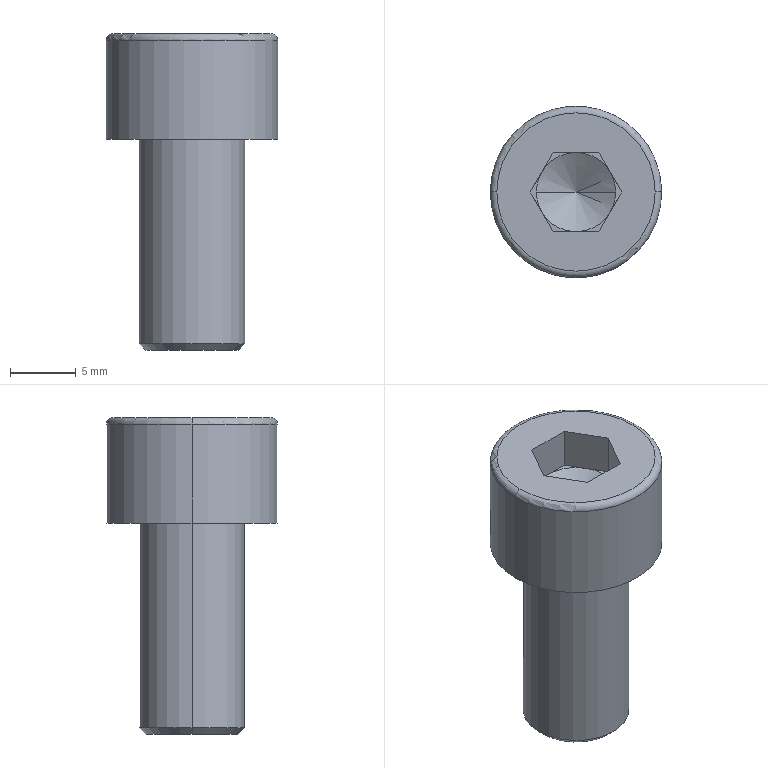Part | NX | features BREP 1 | 1 solid | 25 faces | box 13 x 13 x 24 mm | volume 1747 mm3 | plane 15 | cone 4 | cylinder 4 | torus 2 | commonest cylinder face diameters 8 x2 13 x2
STEP:
#1=CARTESIAN_POINT('',(0.,0.,3.148));
#2=VERTEX_POINT('',#1);
#3=CARTESIAN_POINT('',(-3.,0.,4.88));
#4=VERTEX_POINT('',#3);
#5=CARTESIAN_POINT('',(-3.,0.,4.88));
#6=DIRECTION('',(-0.866,0.,0.5));
#7=VECTOR('',#6,1000.);
#8=LINE('',#5,#7);
#9=EDGE_CURVE('',#2,#4,#8,.T.);
#10=ORIENTED_EDGE('',*,*,#9,.F.);
#11=CARTESIAN_POINT('',(3.,0.,4.88));
#12=VERTEX_POINT('',#11);
#13=CARTESIAN_POINT('',(3.,0.,4.88));
#14=DIRECTION('',(0.866,0.,0.5));
#15=VECTOR('',#14,1000.);
#16=LINE('',#13,#15);
#17=EDGE_CURVE('',#2,#12,#16,.T.);
#18=ORIENTED_EDGE('',*,*,#17,.T.);
#19=CARTESIAN_POINT('',(2.598,1.5,4.88));
#20=VERTEX_POINT('',#19);
#21=CARTESIAN_POINT('',(0.,0.,4.88));
#22=DIRECTION('',(0.,0.,1.));
#23=DIRECTION('',(1.,0.,0.));
#24=AXIS2_PLACEMENT_3D('',#21,#22,#23);
#25=CIRCLE('',#24,3.);
#26=EDGE_CURVE('',#12,#20,#25,.T.);
#27=ORIENTED_EDGE('',*,*,#26,.T.);
#28=CARTESIAN_POINT('',(0.,3.,4.88));
#29=VERTEX_POINT('',#28);
#30=CARTESIAN_POINT('',(0.,0.,4.88));
#31=DIRECTION('',(0.,0.,1.));
#32=DIRECTION('',(1.,0.,0.));
#33=AXIS2_PLACEMENT_3D('',#30,#31,#32);
#34=CIRCLE('',#33,3.);
#35=EDGE_CURVE('',#20,#29,#34,.T.);
#36=ORIENTED_EDGE('',*,*,#35,.T.);
#37=CARTESIAN_POINT('',(-2.598,1.5,4.88));
#38=VERTEX_POINT('',#37);
#39=CARTESIAN_POINT('',(0.,0.,4.88));
#40=DIRECTION('',(0.,0.,-1.));
#41=DIRECTION('',(-1.,0.,0.));
#42=AXIS2_PLACEMENT_3D('',#39,#40,#41);
#43=CIRCLE('',#42,3.);
#44=EDGE_CURVE('',#38,#29,#43,.T.);
#45=ORIENTED_EDGE('',*,*,#44,.F.);
#46=CARTESIAN_POINT('',(0.,0.,4.88));
#47=DIRECTION('',(0.,0.,1.));
#48=DIRECTION('',(1.,0.,0.));
#49=AXIS2_PLACEMENT_3D('',#46,#47,#48);
#50=CIRCLE('',#49,3.);
#51=EDGE_CURVE('',#38,#4,#50,.T.);
#52=ORIENTED_EDGE('',*,*,#51,.T.);
#53=EDGE_LOOP('',(#10,#18,#27,#36,#45,#52));
#54=FACE_BOUND('',#53,.T.);
#55=CARTESIAN_POINT('',(0.,0.,4.88));
#56=DIRECTION('',(0.,0.,1.));
#57=DIRECTION('',(-1.,0.,0.));
#58=AXIS2_PLACEMENT_3D('',#55,#56,#57);
#59=CONICAL_SURFACE('',#58,3.,1.047);
#60=ADVANCED_FACE('',(#54),#59,.F.);
#61=CARTESIAN_POINT('',(-3.5,0.,-16.));
#62=VERTEX_POINT('',#61);
#63=CARTESIAN_POINT('',(3.5,0.,-16.));
#64=VERTEX_POINT('',#63);
#65=CARTESIAN_POINT('',(0.,0.,-16.));
#66=DIRECTION('',(0.,0.,1.));
#67=DIRECTION('',(-1.,0.,0.));
#68=AXIS2_PLACEMENT_3D('',#65,#66,#67);
#69=CIRCLE('',#68,3.5);
#70=EDGE_CURVE('',#62,#64,#69,.T.);
#71=ORIENTED_EDGE('',*,*,#70,.T.);
#72=CARTESIAN_POINT('',(4.,0.,-15.5));
#73=VERTEX_POINT('',#72);
#74=CARTESIAN_POINT('',(4.,0.,-15.5));
#75=DIRECTION('',(0.7071,0.,0.7071));
#76=VECTOR('',#75,1000.);
#77=LINE('',#74,#76);
#78=EDGE_CURVE('',#64,#73,#77,.T.);
#79=ORIENTED_EDGE('',*,*,#78,.T.);
#80=CARTESIAN_POINT('',(-4.,0.,-15.5));
#81=VERTEX_POINT('',#80);
#82=CARTESIAN_POINT('',(0.,0.,-15.5));
#83=DIRECTION('',(0.,0.,-1.));
#84=DIRECTION('',(-1.,0.,0.));
#85=AXIS2_PLACEMENT_3D('',#82,#83,#84);
#86=CIRCLE('',#85,4.);
#87=EDGE_CURVE('',#73,#81,#86,.T.);
#88=ORIENTED_EDGE('',*,*,#87,.T.);
#89=CARTESIAN_POINT('',(-4.,0.,-15.5));
#90=DIRECTION('',(-0.7071,0.,0.7071));
#91=VECTOR('',#90,1000.);
#92=LINE('',#89,#91);
#93=EDGE_CURVE('',#62,#81,#92,.T.);
#94=ORIENTED_EDGE('',*,*,#93,.F.);
#95=EDGE_LOOP('',(#71,#79,#88,#94));
#96=FACE_BOUND('',#95,.T.);
#97=CARTESIAN_POINT('',(0.,0.,-15.5));
#98=DIRECTION('',(0.,0.,1.));
#99=DIRECTION('',(-1.,0.,0.));
#100=AXIS2_PLACEMENT_3D('',#97,#98,#99);
#101=CONICAL_SURFACE('',#100,4.,0.7854);
#102=ADVANCED_FACE('',(#96),#101,.T.);
#103=CARTESIAN_POINT('',(6.,0.,8.));
#104=VERTEX_POINT('',#103);
#105=CARTESIAN_POINT('',(-6.,0.,8.));
#106=VERTEX_POINT('',#105);
#107=CARTESIAN_POINT('',(0.,0.,8.));
#108=DIRECTION('',(0.,0.,-1.));
#109=DIRECTION('',(1.,0.,0.));
#110=AXIS2_PLACEMENT_3D('',#107,#108,#109);
#111=CIRCLE('',#110,6.);
#112=EDGE_CURVE('',#104,#106,#111,.T.);
#113=ORIENTED_EDGE('',*,*,#112,.T.);
#114=CARTESIAN_POINT('',(-6.5,0.,7.5));
#115=VERTEX_POINT('',#114);
#116=CARTESIAN_POINT('',(-6.,0.,7.5));
#117=DIRECTION('',(0.,-1.,0.));
#118=DIRECTION('',(1.,0.,0.));
#119=AXIS2_PLACEMENT_3D('',#116,#117,#118);
#120=CIRCLE('',#119,0.5);
#121=EDGE_CURVE('',#115,#106,#120,.F.);
#122=ORIENTED_EDGE('',*,*,#121,.F.);
#123=CARTESIAN_POINT('',(6.5,0.,7.5));
#124=VERTEX_POINT('',#123);
#125=CARTESIAN_POINT('',(0.,0.,7.5));
#126=DIRECTION('',(0.,0.,1.));
#127=DIRECTION('',(1.,0.,0.));
#128=AXIS2_PLACEMENT_3D('',#125,#126,#127);
#129=CIRCLE('',#128,6.5);
#130=EDGE_CURVE('',#115,#124,#129,.T.);
#131=ORIENTED_EDGE('',*,*,#130,.T.);
#132=CARTESIAN_POINT('',(6.,0.,7.5));
#133=DIRECTION('',(0.,1.,0.));
#134=DIRECTION('',(0.,0.,1.));
#135=AXIS2_PLACEMENT_3D('',#132,#133,#134);
#136=CIRCLE('',#135,0.5);
#137=EDGE_CURVE('',#124,#104,#136,.F.);
#138=ORIENTED_EDGE('',*,*,#137,.T.);
#139=EDGE_LOOP('',(#113,#122,#131,#138));
#140=FACE_BOUND('',#139,.T.);
#141=CARTESIAN_POINT('',(0.,0.,7.5));
#142=DIRECTION('',(0.,0.,-1.));
#143=DIRECTION('',(1.,0.,0.));
#144=AXIS2_PLACEMENT_3D('',#141,#142,#143);
#145=TOROIDAL_SURFACE('',#144,6.,0.5);
#146=ADVANCED_FACE('',(#140),#145,.T.);
#147=ORIENTED_EDGE('',*,*,#87,.F.);
#148=CARTESIAN_POINT('',(4.,0.,0.));
#149=VERTEX_POINT('',#148);
#150=CARTESIAN_POINT('',(4.,0.,-16.));
#151=DIRECTION('',(0.,0.,1.));
#152=VECTOR('',#151,1000.);
#153=LINE('',#150,#152);
#154=EDGE_CURVE('',#73,#149,#153,.T.);
#155=ORIENTED_EDGE('',*,*,#154,.T.);
#156=CARTESIAN_POINT('',(-4.,0.,0.));
#157=VERTEX_POINT('',#156);
#158=CARTESIAN_POINT('',(0.,0.,0.));
#159=DIRECTION('',(0.,0.,1.));
#160=DIRECTION('',(1.,0.,0.));
#161=AXIS2_PLACEMENT_3D('',#158,#159,#160);
#162=CIRCLE('',#161,4.);
#163=EDGE_CURVE('',#157,#149,#162,.T.);
#164=ORIENTED_EDGE('',*,*,#163,.F.);
#165=CARTESIAN_POINT('',(-4.,0.,-16.));
#166=DIRECTION('',(0.,0.,1.));
#167=VECTOR('',#166,1000.);
#168=LINE('',#165,#167);
#169=EDGE_CURVE('',#81,#157,#168,.T.);
#170=ORIENTED_EDGE('',*,*,#169,.F.);
#171=EDGE_LOOP('',(#147,#155,#164,#170));
#172=FACE_BOUND('',#171,.T.);
#173=CARTESIAN_POINT('',(0.,0.,-16.));
#174=DIRECTION('',(0.,0.,1.));
#175=DIRECTION('',(-1.,0.,0.));
#176=AXIS2_PLACEMENT_3D('',#173,#174,#175);
#177=CYLINDRICAL_SURFACE('',#176,4.);
#178=ADVANCED_FACE('',(#172),#177,.T.);
#179=ORIENTED_EDGE('',*,*,#130,.F.);
#180=CARTESIAN_POINT('',(-6.5,0.,0.));
#181=VERTEX_POINT('',#180);
#182=CARTESIAN_POINT('',(-6.5,0.,8.));
#183=DIRECTION('',(0.,0.,-1.));
#184=VECTOR('',#183,1000.);
#185=LINE('',#182,#184);
#186=EDGE_CURVE('',#181,#115,#185,.F.);
#187=ORIENTED_EDGE('',*,*,#186,.F.);
#188=CARTESIAN_POINT('',(6.5,0.,0.));
#189=VERTEX_POINT('',#188);
#190=CARTESIAN_POINT('',(0.,0.,0.));
#191=DIRECTION('',(0.,0.,1.));
#192=DIRECTION('',(1.,0.,0.));
#193=AXIS2_PLACEMENT_3D('',#190,#191,#192);
#194=CIRCLE('',#193,6.5);
#195=EDGE_CURVE('',#181,#189,#194,.T.);
#196=ORIENTED_EDGE('',*,*,#195,.T.);
#197=CARTESIAN_POINT('',(6.5,0.,8.));
#198=DIRECTION('',(0.,0.,-1.));
#199=VECTOR('',#198,1000.);
#200=LINE('',#197,#199);
#201=EDGE_CURVE('',#189,#124,#200,.F.);
#202=ORIENTED_EDGE('',*,*,#201,.T.);
#203=EDGE_LOOP('',(#179,#187,#196,#202));
#204=FACE_BOUND('',#203,.T.);
#205=CARTESIAN_POINT('',(0.,0.,8.));
#206=DIRECTION('',(0.,0.,-1.));
#207=DIRECTION('',(1.,0.,0.));
#208=AXIS2_PLACEMENT_3D('',#205,#206,#207);
#209=CYLINDRICAL_SURFACE('',#208,6.5);
#210=ADVANCED_FACE('',(#204),#209,.T.);
#211=CARTESIAN_POINT('',(1.732,3.,4.88));
#212=VERTEX_POINT('',#211);
#213=CARTESIAN_POINT('',(3.464,0.,4.88));
#214=DIRECTION('',(-0.5,0.866,0.));
#215=VECTOR('',#214,1000.);
#216=LINE('',#213,#215);
#217=EDGE_CURVE('',#20,#212,#216,.T.);
#218=ORIENTED_EDGE('',*,*,#217,.T.);
#219=CARTESIAN_POINT('',(1.732,3.,4.88));
#220=DIRECTION('',(-1.,0.,0.));
#221=VECTOR('',#220,1000.);
#222=LINE('',#219,#221);
#223=EDGE_CURVE('',#212,#29,#222,.T.);
#224=ORIENTED_EDGE('',*,*,#223,.T.);
#225=ORIENTED_EDGE('',*,*,#35,.F.);
#226=EDGE_LOOP('',(#218,#224,#225));
#227=FACE_BOUND('',#226,.T.);
#228=CARTESIAN_POINT('',(0.,0.,4.88));
#229=DIRECTION('',(0.,0.,-1.));
#230=DIRECTION('',(0.,-1.,0.));
#231=AXIS2_PLACEMENT_3D('',#228,#229,#230);
#232=PLANE('',#231);
#233=ADVANCED_FACE('',(#227),#232,.F.);
#234=CARTESIAN_POINT('',(-1.732,3.,4.88));
#235=VERTEX_POINT('',#234);
#236=CARTESIAN_POINT('',(1.732,3.,4.88));
#237=DIRECTION('',(-1.,0.,0.));
#238=VECTOR('',#237,1000.);
#239=LINE('',#236,#238);
#240=EDGE_CURVE('',#29,#235,#239,.T.);
#241=ORIENTED_EDGE('',*,*,#240,.T.);
#242=CARTESIAN_POINT('',(-1.732,3.,4.88));
#243=DIRECTION('',(-0.5,-0.866,0.));
#244=VECTOR('',#243,1000.);
#245=LINE('',#242,#244);
#246=EDGE_CURVE('',#235,#38,#245,.T.);
#247=ORIENTED_EDGE('',*,*,#246,.T.);
#248=ORIENTED_EDGE('',*,*,#44,.T.);
#249=EDGE_LOOP('',(#241,#247,#248));
#250=FACE_BOUND('',#249,.T.);
#251=CARTESIAN_POINT('',(0.,0.,4.88));
#252=DIRECTION('',(0.,0.,-1.));
#253=DIRECTION('',(0.,-1.,0.));
#254=AXIS2_PLACEMENT_3D('',#251,#252,#253);
#255=PLANE('',#254);
#256=ADVANCED_FACE('',(#250),#255,.F.);
#257=CARTESIAN_POINT('',(-3.464,0.,4.88));
#258=VERTEX_POINT('',#257);
#259=CARTESIAN_POINT('',(-1.732,3.,4.88));
#260=DIRECTION('',(-0.5,-0.866,0.));
#261=VECTOR('',#260,1000.);
#262=LINE('',#259,#261);
#263=EDGE_CURVE('',#38,#258,#262,.T.);
#264=ORIENTED_EDGE('',*,*,#263,.T.);
#265=CARTESIAN_POINT('',(-2.598,-1.5,4.88));
#266=VERTEX_POINT('',#265);
#267=CARTESIAN_POINT('',(-3.464,0.,4.88));
#268=DIRECTION('',(0.5,-0.866,0.));
#269=VECTOR('',#268,1000.);
#270=LINE('',#267,#269);
#271=EDGE_CURVE('',#258,#266,#270,.T.);
#272=ORIENTED_EDGE('',*,*,#271,.T.);
#273=CARTESIAN_POINT('',(0.,0.,4.88));
#274=DIRECTION('',(0.,0.,1.));
#275=DIRECTION('',(1.,0.,0.));
#276=AXIS2_PLACEMENT_3D('',#273,#274,#275);
#277=CIRCLE('',#276,3.);
#278=EDGE_CURVE('',#4,#266,#277,.T.);
#279=ORIENTED_EDGE('',*,*,#278,.F.);
#280=ORIENTED_EDGE('',*,*,#51,.F.);
#281=EDGE_LOOP('',(#264,#272,#279,#280));
#282=FACE_BOUND('',#281,.T.);
#283=CARTESIAN_POINT('',(0.,0.,4.88));
#284=DIRECTION('',(0.,0.,-1.));
#285=DIRECTION('',(0.,-1.,0.));
#286=AXIS2_PLACEMENT_3D('',#283,#284,#285);
#287=PLANE('',#286);
#288=ADVANCED_FACE('',(#282),#287,.F.);
#289=CARTESIAN_POINT('',(-1.732,-3.,4.88));
#290=VERTEX_POINT('',#289);
#291=CARTESIAN_POINT('',(-3.464,0.,4.88));
#292=DIRECTION('',(0.5,-0.866,0.));
#293=VECTOR('',#292,1000.);
#294=LINE('',#291,#293);
#295=EDGE_CURVE('',#266,#290,#294,.T.);
#296=ORIENTED_EDGE('',*,*,#295,.T.);
#297=CARTESIAN_POINT('',(0.,-3.,4.88));
#298=VERTEX_POINT('',#297);
#299=CARTESIAN_POINT('',(-1.732,-3.,4.88));
#300=DIRECTION('',(1.,0.,0.));
#301=VECTOR('',#300,1000.);
#302=LINE('',#299,#301);
#303=EDGE_CURVE('',#290,#298,#302,.T.);
#304=ORIENTED_EDGE('',*,*,#303,.T.);
#305=CARTESIAN_POINT('',(0.,0.,4.88));
#306=DIRECTION('',(0.,0.,1.));
#307=DIRECTION('',(1.,0.,0.));
#308=AXIS2_PLACEMENT_3D('',#305,#306,#307);
#309=CIRCLE('',#308,3.);
#310=EDGE_CURVE('',#266,#298,#309,.T.);
#311=ORIENTED_EDGE('',*,*,#310,.F.);
#312=EDGE_LOOP('',(#296,#304,#311));
#313=FACE_BOUND('',#312,.T.);
#314=CARTESIAN_POINT('',(0.,0.,4.88));
#315=DIRECTION('',(0.,0.,-1.));
#316=DIRECTION('',(0.,-1.,0.));
#317=AXIS2_PLACEMENT_3D('',#314,#315,#316);
#318=PLANE('',#317);
#319=ADVANCED_FACE('',(#313),#318,.F.);
#320=CARTESIAN_POINT('',(1.732,-3.,4.88));
#321=VERTEX_POINT('',#320);
#322=CARTESIAN_POINT('',(-1.732,-3.,4.88));
#323=DIRECTION('',(1.,0.,0.));
#324=VECTOR('',#323,1000.);
#325=LINE('',#322,#324);
#326=EDGE_CURVE('',#298,#321,#325,.T.);
#327=ORIENTED_EDGE('',*,*,#326,.T.);
#328=CARTESIAN_POINT('',(2.598,-1.5,4.88));
#329=VERTEX_POINT('',#328);
#330=CARTESIAN_POINT('',(1.732,-3.,4.88));
#331=DIRECTION('',(0.5,0.866,0.));
#332=VECTOR('',#331,1000.);
#333=LINE('',#330,#332);
#334=EDGE_CURVE('',#321,#329,#333,.T.);
#335=ORIENTED_EDGE('',*,*,#334,.T.);
#336=CARTESIAN_POINT('',(0.,0.,4.88));
#337=DIRECTION('',(0.,0.,1.));
#338=DIRECTION('',(1.,0.,0.));
#339=AXIS2_PLACEMENT_3D('',#336,#337,#338);
#340=CIRCLE('',#339,3.);
#341=EDGE_CURVE('',#298,#329,#340,.T.);
#342=ORIENTED_EDGE('',*,*,#341,.F.);
#343=EDGE_LOOP('',(#327,#335,#342));
#344=FACE_BOUND('',#343,.T.);
#345=CARTESIAN_POINT('',(0.,0.,4.88));
#346=DIRECTION('',(0.,0.,-1.));
#347=DIRECTION('',(0.,-1.,0.));
#348=AXIS2_PLACEMENT_3D('',#345,#346,#347);
#349=PLANE('',#348);
#350=ADVANCED_FACE('',(#344),#349,.F.);
#351=ORIENTED_EDGE('',*,*,#112,.F.);
#352=CARTESIAN_POINT('',(0.,0.,8.));
#353=DIRECTION('',(0.,0.,-1.));
#354=DIRECTION('',(1.,0.,0.));
#355=AXIS2_PLACEMENT_3D('',#352,#353,#354);
#356=CIRCLE('',#355,6.);
#357=EDGE_CURVE('',#106,#104,#356,.T.);
#358=ORIENTED_EDGE('',*,*,#357,.F.);
#359=EDGE_LOOP('',(#351,#358));
#360=FACE_BOUND('',#359,.T.);
#361=CARTESIAN_POINT('',(3.464,0.,8.));
#362=VERTEX_POINT('',#361);
#363=CARTESIAN_POINT('',(1.732,3.,8.));
#364=VERTEX_POINT('',#363);
#365=CARTESIAN_POINT('',(3.464,0.,8.));
#366=DIRECTION('',(-0.5,0.866,0.));
#367=VECTOR('',#366,1000.);
#368=LINE('',#365,#367);
#369=EDGE_CURVE('',#362,#364,#368,.T.);
#370=ORIENTED_EDGE('',*,*,#369,.F.);
#371=CARTESIAN_POINT('',(1.732,-3.,8.));
#372=VERTEX_POINT('',#371);
#373=CARTESIAN_POINT('',(1.732,-3.,8.));
#374=DIRECTION('',(0.5,0.866,0.));
#375=VECTOR('',#374,1000.);
#376=LINE('',#373,#375);
#377=EDGE_CURVE('',#372,#362,#376,.T.);
#378=ORIENTED_EDGE('',*,*,#377,.F.);
#379=CARTESIAN_POINT('',(-1.732,-3.,8.));
#380=VERTEX_POINT('',#379);
#381=CARTESIAN_POINT('',(-1.732,-3.,8.));
#382=DIRECTION('',(1.,0.,0.));
#383=VECTOR('',#382,1000.);
#384=LINE('',#381,#383);
#385=EDGE_CURVE('',#380,#372,#384,.T.);
#386=ORIENTED_EDGE('',*,*,#385,.F.);
#387=CARTESIAN_POINT('',(-3.464,0.,8.));
#388=VERTEX_POINT('',#387);
#389=CARTESIAN_POINT('',(-3.464,0.,8.));
#390=DIRECTION('',(0.5,-0.866,0.));
#391=VECTOR('',#390,1000.);
#392=LINE('',#389,#391);
#393=EDGE_CURVE('',#388,#380,#392,.T.);
#394=ORIENTED_EDGE('',*,*,#393,.F.);
#395=CARTESIAN_POINT('',(-1.732,3.,8.));
#396=VERTEX_POINT('',#395);
#397=CARTESIAN_POINT('',(-1.732,3.,8.));
#398=DIRECTION('',(-0.5,-0.866,0.));
#399=VECTOR('',#398,1000.);
#400=LINE('',#397,#399);
#401=EDGE_CURVE('',#396,#388,#400,.T.);
#402=ORIENTED_EDGE('',*,*,#401,.F.);
#403=CARTESIAN_POINT('',(1.732,3.,8.));
#404=DIRECTION('',(-1.,0.,0.));
#405=VECTOR('',#404,1000.);
#406=LINE('',#403,#405);
#407=EDGE_CURVE('',#364,#396,#406,.T.);
#408=ORIENTED_EDGE('',*,*,#407,.F.);
#409=EDGE_LOOP('',(#370,#378,#386,#394,#402,#408));
#410=FACE_BOUND('',#409,.T.);
#411=CARTESIAN_POINT('',(0.,0.,8.));
#412=DIRECTION('',(0.,0.,-1.));
#413=DIRECTION('',(0.,-1.,0.));
#414=AXIS2_PLACEMENT_3D('',#411,#412,#413);
#415=PLANE('',#414);
#416=ADVANCED_FACE('',(#360,#410),#415,.F.);
#417=ORIENTED_EDGE('',*,*,#186,.T.);
#418=CARTESIAN_POINT('',(0.,0.,7.5));
#419=DIRECTION('',(0.,0.,1.));
#420=DIRECTION('',(1.,0.,0.));
#421=AXIS2_PLACEMENT_3D('',#418,#419,#420);
#422=CIRCLE('',#421,6.5);
#423=EDGE_CURVE('',#124,#115,#422,.T.);
#424=ORIENTED_EDGE('',*,*,#423,.F.);
#425=ORIENTED_EDGE('',*,*,#201,.F.);
#426=CARTESIAN_POINT('',(0.,0.,0.));
#427=DIRECTION('',(0.,0.,1.));
#428=DIRECTION('',(1.,0.,0.));
#429=AXIS2_PLACEMENT_3D('',#426,#427,#428);
#430=CIRCLE('',#429,6.5);
#431=EDGE_CURVE('',#189,#181,#430,.T.);
#432=ORIENTED_EDGE('',*,*,#431,.T.);
#433=EDGE_LOOP('',(#417,#424,#425,#432));
#434=FACE_BOUND('',#433,.T.);
#435=CARTESIAN_POINT('',(0.,0.,8.));
#436=DIRECTION('',(0.,0.,-1.));
#437=DIRECTION('',(1.,0.,0.));
#438=AXIS2_PLACEMENT_3D('',#435,#436,#437);
#439=CYLINDRICAL_SURFACE('',#438,6.5);
#440=ADVANCED_FACE('',(#434),#439,.T.);
#441=ORIENTED_EDGE('',*,*,#431,.F.);
#442=ORIENTED_EDGE('',*,*,#195,.F.);
#443=EDGE_LOOP('',(#441,#442));
#444=FACE_BOUND('',#443,.T.);
#445=ORIENTED_EDGE('',*,*,#163,.T.);
#446=CARTESIAN_POINT('',(0.,0.,0.));
#447=DIRECTION('',(0.,0.,1.));
#448=DIRECTION('',(1.,0.,0.));
#449=AXIS2_PLACEMENT_3D('',#446,#447,#448);
#450=CIRCLE('',#449,4.);
#451=EDGE_CURVE('',#149,#157,#450,.T.);
#452=ORIENTED_EDGE('',*,*,#451,.T.);
#453=EDGE_LOOP('',(#445,#452));
#454=FACE_BOUND('',#453,.T.);
#455=CARTESIAN_POINT('',(0.,0.,0.));
#456=DIRECTION('',(0.,0.,-1.));
#457=DIRECTION('',(0.,-1.,0.));
#458=AXIS2_PLACEMENT_3D('',#455,#456,#457);
#459=PLANE('',#458);
#460=ADVANCED_FACE('',(#444,#454),#459,.T.);
#461=ORIENTED_EDGE('',*,*,#154,.F.);
#462=CARTESIAN_POINT('',(0.,0.,-15.5));
#463=DIRECTION('',(0.,0.,-1.));
#464=DIRECTION('',(-1.,0.,0.));
#465=AXIS2_PLACEMENT_3D('',#462,#463,#464);
#466=CIRCLE('',#465,4.);
#467=EDGE_CURVE('',#81,#73,#466,.T.);
#468=ORIENTED_EDGE('',*,*,#467,.F.);
#469=ORIENTED_EDGE('',*,*,#169,.T.);
#470=ORIENTED_EDGE('',*,*,#451,.F.);
#471=EDGE_LOOP('',(#461,#468,#469,#470));
#472=FACE_BOUND('',#471,.T.);
#473=CARTESIAN_POINT('',(0.,0.,-16.));
#474=DIRECTION('',(0.,0.,1.));
#475=DIRECTION('',(-1.,0.,0.));
#476=AXIS2_PLACEMENT_3D('',#473,#474,#475);
#477=CYLINDRICAL_SURFACE('',#476,4.);
#478=ADVANCED_FACE('',(#472),#477,.T.);
#479=ORIENTED_EDGE('',*,*,#70,.F.);
#480=CARTESIAN_POINT('',(0.,0.,-16.));
#481=DIRECTION('',(0.,0.,1.));
#482=DIRECTION('',(-1.,0.,0.));
#483=AXIS2_PLACEMENT_3D('',#480,#481,#482);
#484=CIRCLE('',#483,3.5);
#485=EDGE_CURVE('',#64,#62,#484,.T.);
#486=ORIENTED_EDGE('',*,*,#485,.F.);
#487=EDGE_LOOP('',(#479,#486));
#488=FACE_BOUND('',#487,.T.);
#489=CARTESIAN_POINT('',(0.,0.,-16.));
#490=DIRECTION('',(0.,0.,1.));
#491=DIRECTION('',(1.,0.,0.));
#492=AXIS2_PLACEMENT_3D('',#489,#490,#491);
#493=PLANE('',#492);
#494=ADVANCED_FACE('',(#488),#493,.F.);
#495=ORIENTED_EDGE('',*,*,#121,.T.);
#496=ORIENTED_EDGE('',*,*,#357,.T.);
#497=ORIENTED_EDGE('',*,*,#137,.F.);
#498=ORIENTED_EDGE('',*,*,#423,.T.);
#499=EDGE_LOOP('',(#495,#496,#497,#498));
#500=FACE_BOUND('',#499,.T.);
#501=CARTESIAN_POINT('',(0.,0.,7.5));
#502=DIRECTION('',(0.,0.,-1.));
#503=DIRECTION('',(1.,0.,0.));
#504=AXIS2_PLACEMENT_3D('',#501,#502,#503);
#505=TOROIDAL_SURFACE('',#504,6.,0.5);
#506=ADVANCED_FACE('',(#500),#505,.T.);
#507=ORIENTED_EDGE('',*,*,#78,.F.);
#508=ORIENTED_EDGE('',*,*,#485,.T.);
#509=ORIENTED_EDGE('',*,*,#93,.T.);
#510=ORIENTED_EDGE('',*,*,#467,.T.);
#511=EDGE_LOOP('',(#507,#508,#509,#510));
#512=FACE_BOUND('',#511,.T.);
#513=CARTESIAN_POINT('',(0.,0.,-15.5));
#514=DIRECTION('',(0.,0.,1.));
#515=DIRECTION('',(-1.,0.,0.));
#516=AXIS2_PLACEMENT_3D('',#513,#514,#515);
#517=CONICAL_SURFACE('',#516,4.,0.7854);
#518=ADVANCED_FACE('',(#512),#517,.T.);
#519=ORIENTED_EDGE('',*,*,#369,.T.);
#520=CARTESIAN_POINT('',(1.732,3.,4.88));
#521=DIRECTION('',(0.,0.,1.));
#522=VECTOR('',#521,1000.);
#523=LINE('',#520,#522);
#524=EDGE_CURVE('',#212,#364,#523,.T.);
#525=ORIENTED_EDGE('',*,*,#524,.F.);
#526=ORIENTED_EDGE('',*,*,#217,.F.);
#527=CARTESIAN_POINT('',(3.464,0.,4.88));
#528=VERTEX_POINT('',#527);
#529=CARTESIAN_POINT('',(3.464,0.,4.88));
#530=DIRECTION('',(-0.5,0.866,0.));
#531=VECTOR('',#530,1000.);
#532=LINE('',#529,#531);
#533=EDGE_CURVE('',#528,#20,#532,.T.);
#534=ORIENTED_EDGE('',*,*,#533,.F.);
#535=CARTESIAN_POINT('',(3.464,0.,4.88));
#536=DIRECTION('',(0.,0.,1.));
#537=VECTOR('',#536,1000.);
#538=LINE('',#535,#537);
#539=EDGE_CURVE('',#528,#362,#538,.T.);
#540=ORIENTED_EDGE('',*,*,#539,.T.);
#541=EDGE_LOOP('',(#519,#525,#526,#534,#540));
#542=FACE_BOUND('',#541,.T.);
#543=CARTESIAN_POINT('',(3.464,0.,4.88));
#544=DIRECTION('',(-0.866,-0.5,0.));
#545=DIRECTION('',(-0.5,0.866,0.));
#546=AXIS2_PLACEMENT_3D('',#543,#544,#545);
#547=PLANE('',#546);
#548=ADVANCED_FACE('',(#542),#547,.T.);
#549=ORIENTED_EDGE('',*,*,#407,.T.);
#550=CARTESIAN_POINT('',(-1.732,3.,4.88));
#551=DIRECTION('',(0.,0.,1.));
#552=VECTOR('',#551,1000.);
#553=LINE('',#550,#552);
#554=EDGE_CURVE('',#235,#396,#553,.T.);
#555=ORIENTED_EDGE('',*,*,#554,.F.);
#556=ORIENTED_EDGE('',*,*,#240,.F.);
#557=ORIENTED_EDGE('',*,*,#223,.F.);
#558=ORIENTED_EDGE('',*,*,#524,.T.);
#559=EDGE_LOOP('',(#549,#555,#556,#557,#558));
#560=FACE_BOUND('',#559,.T.);
#561=CARTESIAN_POINT('',(1.732,3.,4.88));
#562=DIRECTION('',(0.,-1.,0.));
#563=DIRECTION('',(0.,0.,-1.));
#564=AXIS2_PLACEMENT_3D('',#561,#562,#563);
#565=PLANE('',#564);
#566=ADVANCED_FACE('',(#560),#565,.T.);
#567=ORIENTED_EDGE('',*,*,#401,.T.);
#568=CARTESIAN_POINT('',(-3.464,0.,4.88));
#569=DIRECTION('',(0.,0.,1.));
#570=VECTOR('',#569,1000.);
#571=LINE('',#568,#570);
#572=EDGE_CURVE('',#258,#388,#571,.T.);
#573=ORIENTED_EDGE('',*,*,#572,.F.);
#574=ORIENTED_EDGE('',*,*,#263,.F.);
#575=ORIENTED_EDGE('',*,*,#246,.F.);
#576=ORIENTED_EDGE('',*,*,#554,.T.);
#577=EDGE_LOOP('',(#567,#573,#574,#575,#576));
#578=FACE_BOUND('',#577,.T.);
#579=CARTESIAN_POINT('',(-1.732,3.,4.88));
#580=DIRECTION('',(0.866,-0.5,0.));
#581=DIRECTION('',(0.,0.,-1.));
#582=AXIS2_PLACEMENT_3D('',#579,#580,#581);
#583=PLANE('',#582);
#584=ADVANCED_FACE('',(#578),#583,.T.);
#585=ORIENTED_EDGE('',*,*,#393,.T.);
#586=CARTESIAN_POINT('',(-1.732,-3.,4.88));
#587=DIRECTION('',(0.,0.,1.));
#588=VECTOR('',#587,1000.);
#589=LINE('',#586,#588);
#590=EDGE_CURVE('',#290,#380,#589,.T.);
#591=ORIENTED_EDGE('',*,*,#590,.F.);
#592=ORIENTED_EDGE('',*,*,#295,.F.);
#593=ORIENTED_EDGE('',*,*,#271,.F.);
#594=ORIENTED_EDGE('',*,*,#572,.T.);
#595=EDGE_LOOP('',(#585,#591,#592,#593,#594));
#596=FACE_BOUND('',#595,.T.);
#597=CARTESIAN_POINT('',(-3.464,0.,4.88));
#598=DIRECTION('',(0.866,0.5,0.));
#599=DIRECTION('',(0.,0.,-1.));
#600=AXIS2_PLACEMENT_3D('',#597,#598,#599);
#601=PLANE('',#600);
#602=ADVANCED_FACE('',(#596),#601,.T.);
#603=ORIENTED_EDGE('',*,*,#385,.T.);
#604=CARTESIAN_POINT('',(1.732,-3.,4.88));
#605=DIRECTION('',(0.,0.,1.));
#606=VECTOR('',#605,1000.);
#607=LINE('',#604,#606);
#608=EDGE_CURVE('',#321,#372,#607,.T.);
#609=ORIENTED_EDGE('',*,*,#608,.F.);
#610=ORIENTED_EDGE('',*,*,#326,.F.);
#611=ORIENTED_EDGE('',*,*,#303,.F.);
#612=ORIENTED_EDGE('',*,*,#590,.T.);
#613=EDGE_LOOP('',(#603,#609,#610,#611,#612));
#614=FACE_BOUND('',#613,.T.);
#615=CARTESIAN_POINT('',(-1.732,-3.,4.88));
#616=DIRECTION('',(0.,1.,0.));
#617=DIRECTION('',(1.,0.,0.));
#618=AXIS2_PLACEMENT_3D('',#615,#616,#617);
#619=PLANE('',#618);
#620=ADVANCED_FACE('',(#614),#619,.T.);
#621=ORIENTED_EDGE('',*,*,#377,.T.);
#622=ORIENTED_EDGE('',*,*,#539,.F.);
#623=CARTESIAN_POINT('',(1.732,-3.,4.88));
#624=DIRECTION('',(0.5,0.866,0.));
#625=VECTOR('',#624,1000.);
#626=LINE('',#623,#625);
#627=EDGE_CURVE('',#329,#528,#626,.T.);
#628=ORIENTED_EDGE('',*,*,#627,.F.);
#629=ORIENTED_EDGE('',*,*,#334,.F.);
#630=ORIENTED_EDGE('',*,*,#608,.T.);
#631=EDGE_LOOP('',(#621,#622,#628,#629,#630));
#632=FACE_BOUND('',#631,.T.);
#633=CARTESIAN_POINT('',(1.732,-3.,4.88));
#634=DIRECTION('',(-0.866,0.5,0.));
#635=DIRECTION('',(0.,0.,1.));
#636=AXIS2_PLACEMENT_3D('',#633,#634,#635);
#637=PLANE('',#636);
#638=ADVANCED_FACE('',(#632),#637,.T.);
#639=ORIENTED_EDGE('',*,*,#627,.T.);
#640=ORIENTED_EDGE('',*,*,#533,.T.);
#641=ORIENTED_EDGE('',*,*,#26,.F.);
#642=CARTESIAN_POINT('',(0.,0.,4.88));
#643=DIRECTION('',(0.,0.,1.));
#644=DIRECTION('',(1.,0.,0.));
#645=AXIS2_PLACEMENT_3D('',#642,#643,#644);
#646=CIRCLE('',#645,3.);
#647=EDGE_CURVE('',#329,#12,#646,.T.);
#648=ORIENTED_EDGE('',*,*,#647,.F.);
#649=EDGE_LOOP('',(#639,#640,#641,#648));
#650=FACE_BOUND('',#649,.T.);
#651=CARTESIAN_POINT('',(0.,0.,4.88));
#652=DIRECTION('',(0.,0.,-1.));
#653=DIRECTION('',(0.,-1.,0.));
#654=AXIS2_PLACEMENT_3D('',#651,#652,#653);
#655=PLANE('',#654);
#656=ADVANCED_FACE('',(#650),#655,.F.);
#657=ORIENTED_EDGE('',*,*,#17,.F.);
#658=ORIENTED_EDGE('',*,*,#9,.T.);
#659=ORIENTED_EDGE('',*,*,#278,.T.);
#660=ORIENTED_EDGE('',*,*,#310,.T.);
#661=ORIENTED_EDGE('',*,*,#341,.T.);
#662=ORIENTED_EDGE('',*,*,#647,.T.);
#663=EDGE_LOOP('',(#657,#658,#659,#660,#661,#662));
#664=FACE_BOUND('',#663,.T.);
#665=CARTESIAN_POINT('',(0.,0.,4.88));
#666=DIRECTION('',(0.,0.,1.));
#667=DIRECTION('',(-1.,0.,0.));
#668=AXIS2_PLACEMENT_3D('',#665,#666,#667);
#669=CONICAL_SURFACE('',#668,3.,1.047);
#670=ADVANCED_FACE('',(#664),#669,.F.);
#671=CLOSED_SHELL('',(#60,#102,#146,#178,#210,#233,#256,#288,#319,#350,#416,#440,#460,#478,#494,#506,#518,#548,#566,#584,#602,#620,#638,#656,#670));
#672=MANIFOLD_SOLID_BREP('',#671);
#673=(LENGTH_UNIT()NAMED_UNIT(*)SI_UNIT(.MILLI.,.METRE.));
#674=UNCERTAINTY_MEASURE_WITH_UNIT(LENGTH_MEASURE(0.00001),#673,'','');
#675=(NAMED_UNIT(*)PLANE_ANGLE_UNIT()SI_UNIT($,.RADIAN.));
#676=(NAMED_UNIT(*)SI_UNIT($,.STERADIAN.)SOLID_ANGLE_UNIT());
#677=(GEOMETRIC_REPRESENTATION_CONTEXT(3)GLOBAL_UNCERTAINTY_ASSIGNED_CONTEXT((#674))GLOBAL_UNIT_ASSIGNED_CONTEXT((#673,#675,#676))REPRESENTATION_CONTEXT('',''));
#678=ADVANCED_BREP_SHAPE_REPRESENTATION('',(#672),#677);